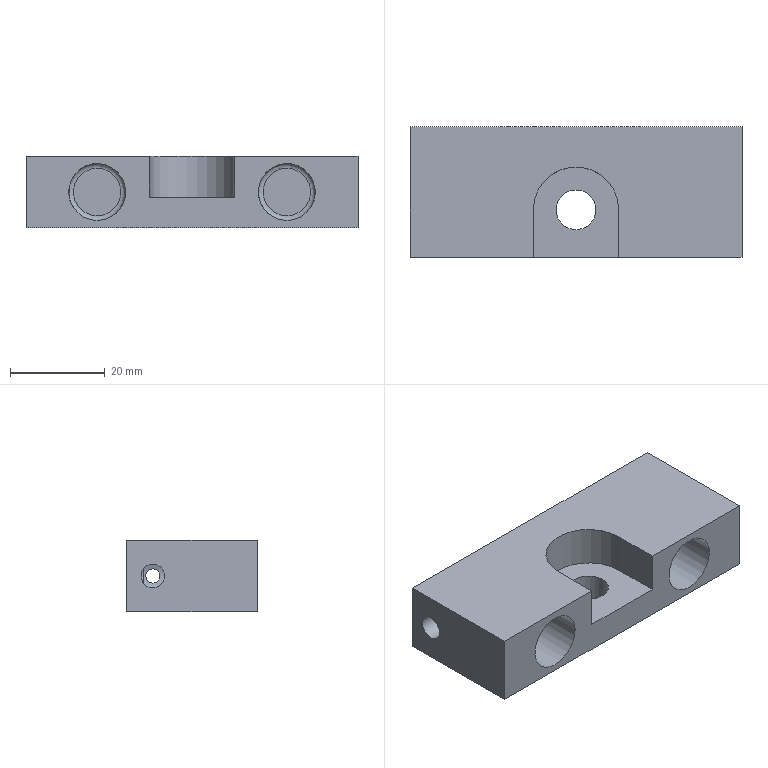NC program | NX | posted with a generic post | part box 70 x 27.5 x 15 mm
Lines 1564 to 1623 of 3352:
(PLANAR_MILL_4 , TOOL : D10-30-D10-75-3T-FINISH)
N3120 T04 M6
N3122 G53
N3124 G17 G0 G90 X-23.75 Y-4. B0. C0. S3000 M3
N3126 G43 Z20. H4
N3128 Z-5.6
N3130 G94 G1 Z-8.6 F600.
N3132 X-13.75
N3134 X-3.75
N3136 G3 X0.25 Y0. R4.
N3138 X-3.75 Y4. R4.
N3140 G1 X-13.75
N3142 X-23.75
N3144 Z-5.6
N3146 G0 Z20.
N3148 Y-4.
N3150 Z-5.6
N3152 G1 Z-8.6
N3154 X-13.75
N3156 X-3.75
N3158 G3 X0.25 Y0. R4.
N3160 X-3.75 Y4. R4.
N3162 G1 X-13.75
N3164 X-23.75
N3166 Z-5.6
N3168 G0 Z20.
(PLANAR_MILL_1 , TOOL : D10-30-D10-75-3T-FINISH)
N3170 X-18.75 Y-43.66
N3172 Z-13.
N3174 G1 Z-16.
N3176 Y-34.999
N3178 Y35.
N3180 G2 X-13.75 Y40. R5.
N3182 G1 X13.75
N3184 G2 X18.75 Y35. R5.
N3186 G1 Y-35.
N3188 G2 X13.75 Y-40. R5.
N3190 G1 X-13.749
N3192 X-22.41
N3194 Z-13.
N3196 G0 Z20.
N3198 X-18.75 Y-43.66
N3200 Z-13.
N3202 G1 Z-16.
N3204 Y-34.999
N3206 Y35.
N3208 G2 X-13.75 Y40. R5.
N3210 G1 X13.75
N3212 G2 X18.75 Y35. R5.
N3214 G1 Y-35.
N3216 G2 X13.75 Y-40. R5.
N3218 G1 X-13.749
N3220 X-22.41
N3222 Z-13.
N3224 G0 Z20.
N3226 M5